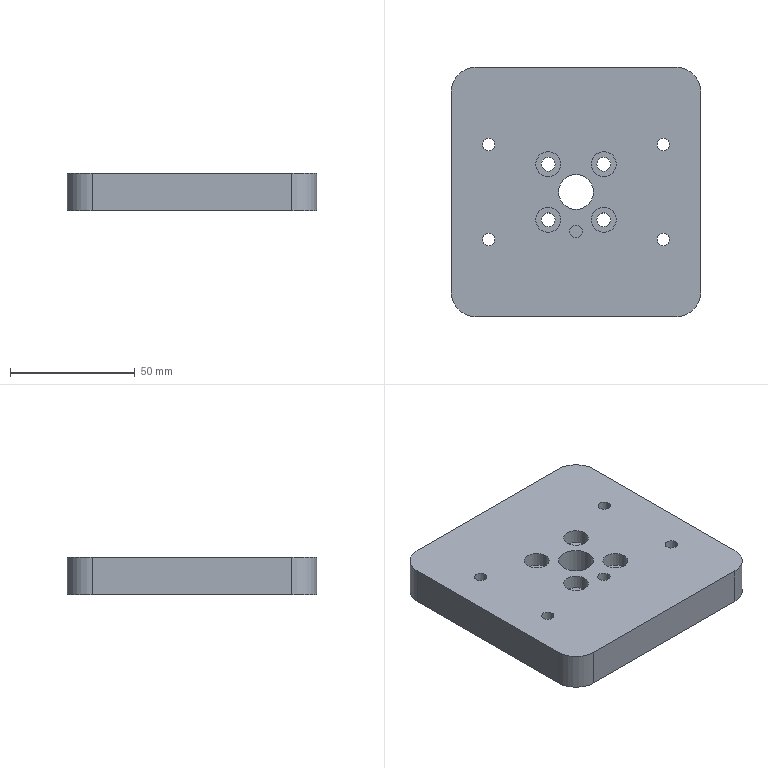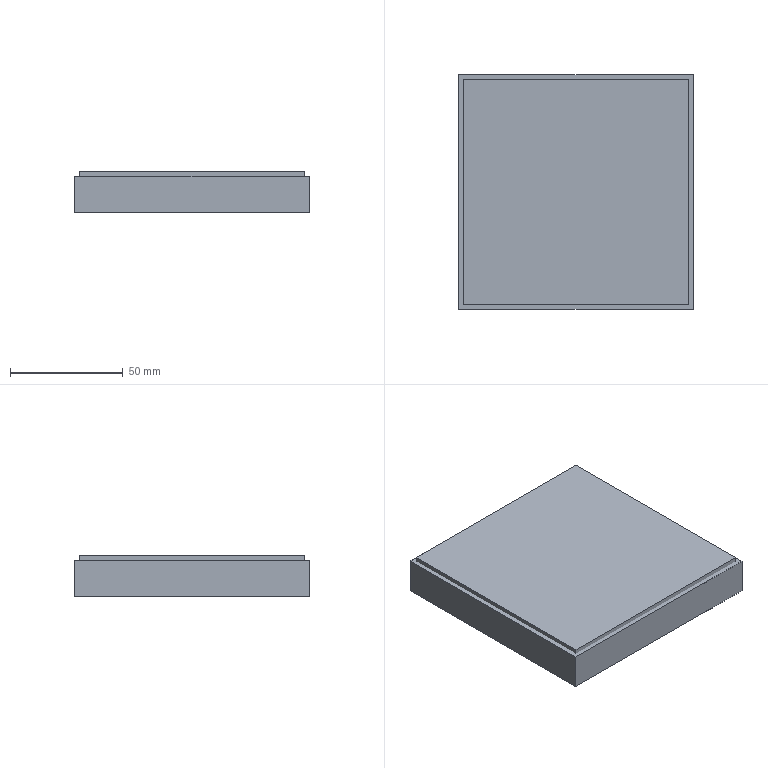CAM job | NX | 3-axis milling, drilling | part box 100 x 100 x 15 mm | stock box 104 x 104 x 18 mm
Tools:
number,name,description,diameter,corner_radius,flute_length,length,flutes
7,D6A45,Milling Tool-5 Parameters,6.0,0.0,50.0,75.0,2
1,D63,Milling Tool-5 Parameters,63.0,0.0,50.0,75.0,2
10,D10,Milling Tool-5 Parameters,10.0,0.0,50.0,75.0,2
15,5.0ZT,Drilling Tool,5.0,0.0,35.0,50.0,2
16,5.5ZT,Drilling Tool,5.5,0.0,35.0,50.0,2
6,D6,Milling Tool-5 Parameters,6.0,0.0,50.0,75.0,2
3,D3,Milling Tool-5 Parameters,3.0,0.0,50.0,75.0,2
Operations:
program,operation,operation_type,tool,method,geometry_group,spindle_rpm,surface_speed,feed_per_tooth,feed_cut,feed_plunge,cut_length_mm,path_length_mm,cut_time_min,machine_time_min
1,FLOOR_WALL_1,VolumeBased25DMillingOperation,D63,METHOD,A,6500.0,1286.0,0.1154,1500.0,100.0,758.797,812.797,0.5059,0.5113
1,ZLEVEL_PROFILE,ZLevelMilling,D10,METHOD,A,9500.0,298.0,0.1842,3500.0,1000.0,7100.688,7172.688,2.062,2.069
1,ZLEVEL_PROFILE_COPY,ZLevelMilling,D10,METHOD,A,9500.0,298.0,0.0789,1500.0,1000.0,422.71,509.71,0.2832,0.2919
1,HOLE_MILLING,CylinderMilling,D10,METHOD,A,9500.0,0.0,0.0,2200.0,100.0,203.595,278.095,0.0925,0.1
1,HOLE_MILLING_COPY,CylinderMilling,D10,METHOD,A,9500.0,0.0,0.0632,1200.0,100.0,43.742,118.242,0.0365,0.0439
1,DRILLING,Operation,D6A45,METHOD,A,5000.0,94.0,0.025,250.0,0.0,40.0,363.244,0.16,0.1923
1,DRILLING_COPY,Operation,5.0ZT,METHOD,A,2000.0,31.0,0.0625,250.0,0.0,84.009,383.318,0.336,0.366
1,DRILLING_COPY_COPY,Operation,5.5ZT,METHOD,A,2000.0,34.0,0.0625,250.0,0.0,78.609,293.644,0.3144,0.3359
1,HOLE_MILLING_1,CylinderMilling,D6,METHOD,A,9500.0,179.0,0.0789,1500.0,100.0,699.183,1026.805,0.4661,0.4989
1,HOLE_MILLING_1_COPY,CylinderMilling,D3,METHOD,A,9500.0,89.0,0.0526,1000.0,100.0,140.615,206.615,0.1406,0.1472
1,PLANAR_MILL,PlanarMilling,D6A45,METHOD,A,9500.0,179.0,0.0658,1250.0,100.0,636.162,1554.901,0.5089,0.6008
1,刀补3,CylinderMilling,D3,METHOD,A,9500.0,89.0,0.0526,1000.0,100.0,31.007,97.007,0.031,0.0376
2,FLOOR_WALL_1_COPY,VolumeBased25DMillingOperation,D63,METHOD,B,6500.0,1286.0,0.1154,1500.0,100.0,2216.391,2521.985,1.478,1.508
2,HOLE_MILLING_COPY_1,CylinderMilling,D10,METHOD,B,9500.0,0.0,0.0,2200.0,100.0,2472.543,2549.043,1.124,1.131
2,PLANAR_MILL_COPY,PlanarMilling,D6A45,METHOD,B,9500.0,179.0,0.0658,1250.0,100.0,642.106,1183.269,0.5137,0.5678
2,PLANAR_MILL_COPY_COPY,PlanarMilling,D6A45,METHOD,B,9500.0,179.0,0.0658,1250.0,100.0,110.295,507.37,0.0882,0.1279
2,刀补10,CylinderMilling,D10,METHOD,B,9500.0,0.0,0.0632,1200.0,100.0,350.373,412.873,0.292,0.2982